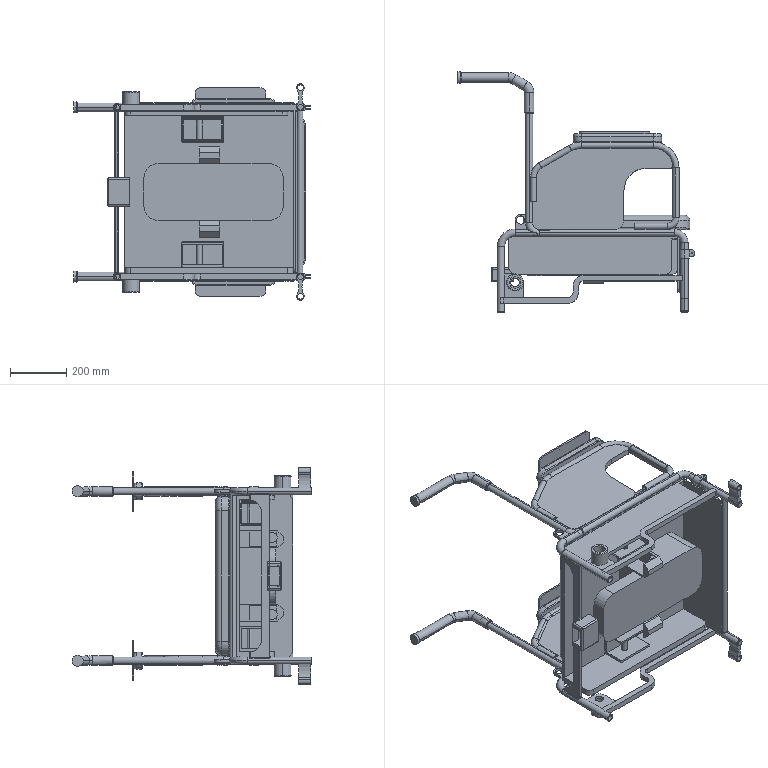Part | SolidWorks | features ICE 30, Fillet 19, MirrorPattern 15, Cut 6, Sweep 4, BossThin 2, Chamfer 2, LPattern 2, MirrorSolid 1 | 1 solid | 916 faces | box 838.639 x 850 x 766 mm | volume 46006837 mm3 | cylinder 385 | plane 373 | torus 126 | spline 16 | cone 10 | sphere 6 | commonest cylinder face diameters 26 x63 20 x56 6 x36 40 x32 22 x26 12 x24